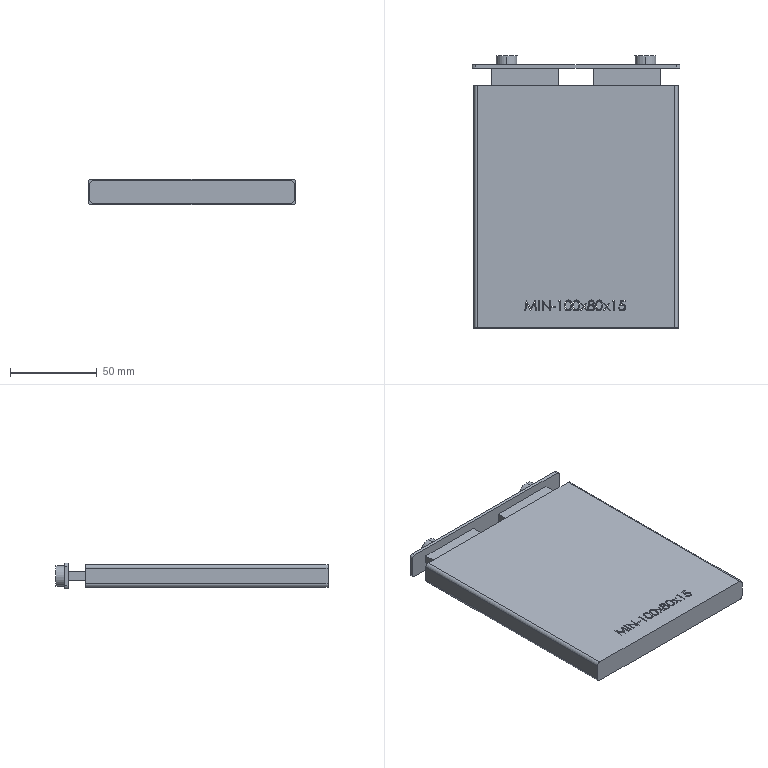Part | STEP file | MIN-Cell | 6 solids | 169 faces | box 120 x 157 x 15 mm | volume 221771 mm3 | plane 105 | spline 52 | cylinder 12 | commonest cylinder face diameters 4 x8 12 x4